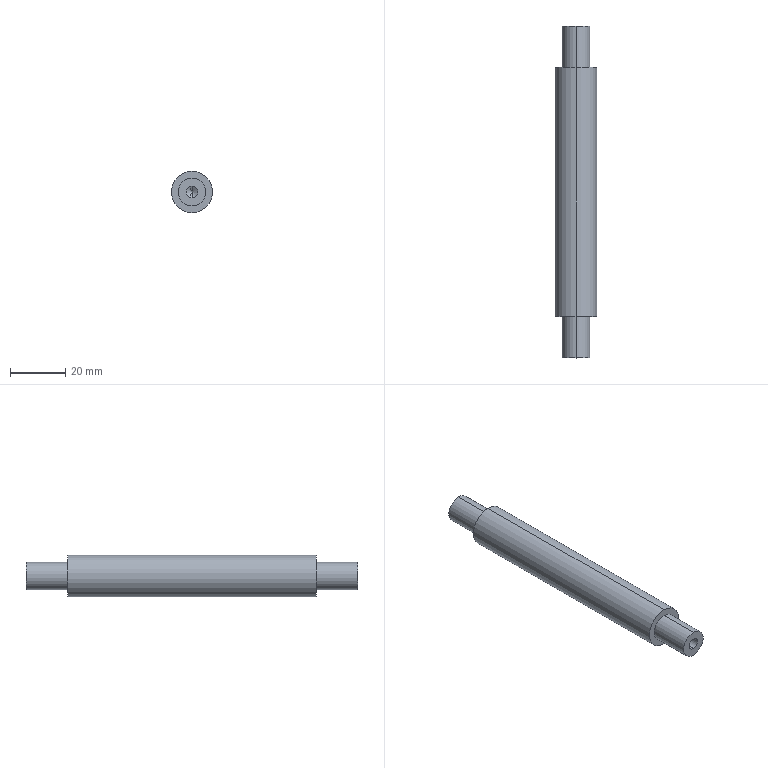Part | STEP file | PN_0006 | 1 solid | 18 faces | box 15 x 120 x 15 mm | volume 17905 mm3 | cylinder 10 | cone 4 | plane 4 | commonest cylinder face diameters 4.2 x4 10 x4 15 x2
STEP:
#1=CARTESIAN_POINT('',(0.,0.,0.));
#2=DIRECTION('',(0.,0.,1.));
#3=DIRECTION('',(1.,0.,0.));
#4=AXIS2_PLACEMENT_3D('',#1,#2,#3);
#5=CARTESIAN_POINT('',(0.,107.6,2.1));
#6=VERTEX_POINT('',#5);
#7=CARTESIAN_POINT('',(0.,120.,2.1));
#8=VERTEX_POINT('',#7);
#9=CARTESIAN_POINT('',(0.,120.,2.1));
#10=DIRECTION('',(0.,1.,0.));
#11=VECTOR('',#10,1.);
#12=LINE('',#9,#11);
#13=CARTESIAN_POINT('',(0.,120.,0.));
#14=DIRECTION('',(0.,1.,0.));
#15=DIRECTION('',(0.,0.,1.));
#16=AXIS2_PLACEMENT_3D('',#13,#14,#15);
#17=CYLINDRICAL_SURFACE('',#16,2.1);
#18=CARTESIAN_POINT('',(6.283,0.));
#19=DIRECTION('',(0.,1.));
#20=VECTOR('',#19,1.);
#21=LINE('',#18,#20);
#22=(GEOMETRIC_REPRESENTATION_CONTEXT(2)PARAMETRIC_REPRESENTATION_CONTEXT()REPRESENTATION_CONTEXT('',''));
#23=DEFINITIONAL_REPRESENTATION('',(#21),#22);
#24=PCURVE('',#17,#23);
#25=CARTESIAN_POINT('',(0.,120.,0.));
#26=DIRECTION('',(0.,1.,0.));
#27=DIRECTION('',(0.,0.,1.));
#28=AXIS2_PLACEMENT_3D('',#25,#26,#27);
#29=CYLINDRICAL_SURFACE('',#28,2.1);
#30=CARTESIAN_POINT('',(0.,0.));
#31=DIRECTION('',(0.,1.));
#32=VECTOR('',#31,1.);
#33=LINE('',#30,#32);
#34=(GEOMETRIC_REPRESENTATION_CONTEXT(2)PARAMETRIC_REPRESENTATION_CONTEXT()REPRESENTATION_CONTEXT('',''));
#35=DEFINITIONAL_REPRESENTATION('',(#33),#34);
#36=PCURVE('',#29,#35);
#37=SURFACE_CURVE('',#12,(#24,#36),.PCURVE_S1.);
#38=EDGE_CURVE('',#6,#8,#37,.T.);
#39=ORIENTED_EDGE('',*,*,#38,.T.);
#40=CARTESIAN_POINT('',(0.,120.,-2.1));
#41=VERTEX_POINT('',#40);
#42=CARTESIAN_POINT('',(0.,120.,0.));
#43=DIRECTION('',(0.,1.,0.));
#44=DIRECTION('',(0.,0.,1.));
#45=AXIS2_PLACEMENT_3D('',#42,#43,#44);
#46=CIRCLE('',#45,2.1);
#47=CARTESIAN_POINT('',(0.,0.));
#48=DIRECTION('',(1.,0.));
#49=VECTOR('',#48,1.);
#50=LINE('',#47,#49);
#51=(GEOMETRIC_REPRESENTATION_CONTEXT(2)PARAMETRIC_REPRESENTATION_CONTEXT()REPRESENTATION_CONTEXT('',''));
#52=DEFINITIONAL_REPRESENTATION('',(#50),#51);
#53=PCURVE('',#17,#52);
#54=CARTESIAN_POINT('',(0.,120.,0.));
#55=DIRECTION('',(0.,1.,0.));
#56=DIRECTION('',(0.,0.,1.));
#57=AXIS2_PLACEMENT_3D('',#54,#55,#56);
#58=PLANE('',#57);
#59=CARTESIAN_POINT('',(0.,0.));
#60=DIRECTION('',(1.,0.));
#61=AXIS2_PLACEMENT_2D('',#59,#60);
#62=CIRCLE('',#61,2.1);
#63=(GEOMETRIC_REPRESENTATION_CONTEXT(2)PARAMETRIC_REPRESENTATION_CONTEXT()REPRESENTATION_CONTEXT('',''));
#64=DEFINITIONAL_REPRESENTATION('',(#62),#63);
#65=PCURVE('',#58,#64);
#66=SURFACE_CURVE('',#46,(#53,#65),.PCURVE_S1.);
#67=EDGE_CURVE('',#41,#8,#66,.T.);
#68=ORIENTED_EDGE('',*,*,#67,.F.);
#69=CARTESIAN_POINT('',(0.,107.6,-2.1));
#70=VERTEX_POINT('',#69);
#71=CARTESIAN_POINT('',(0.,120.,-2.1));
#72=DIRECTION('',(0.,1.,0.));
#73=VECTOR('',#72,1.);
#74=LINE('',#71,#73);
#75=CARTESIAN_POINT('',(3.142,0.));
#76=DIRECTION('',(0.,1.));
#77=VECTOR('',#76,1.);
#78=LINE('',#75,#77);
#79=(GEOMETRIC_REPRESENTATION_CONTEXT(2)PARAMETRIC_REPRESENTATION_CONTEXT()REPRESENTATION_CONTEXT('',''));
#80=DEFINITIONAL_REPRESENTATION('',(#78),#79);
#81=PCURVE('',#17,#80);
#82=CARTESIAN_POINT('',(3.142,0.));
#83=DIRECTION('',(0.,1.));
#84=VECTOR('',#83,1.);
#85=LINE('',#82,#84);
#86=(GEOMETRIC_REPRESENTATION_CONTEXT(2)PARAMETRIC_REPRESENTATION_CONTEXT()REPRESENTATION_CONTEXT('',''));
#87=DEFINITIONAL_REPRESENTATION('',(#85),#86);
#88=PCURVE('',#29,#87);
#89=SURFACE_CURVE('',#74,(#81,#88),.PCURVE_S1.);
#90=EDGE_CURVE('',#70,#41,#89,.T.);
#91=ORIENTED_EDGE('',*,*,#90,.F.);
#92=CARTESIAN_POINT('',(0.,107.6,0.));
#93=DIRECTION('',(0.,1.,0.));
#94=DIRECTION('',(0.,0.,1.));
#95=AXIS2_PLACEMENT_3D('',#92,#93,#94);
#96=CIRCLE('',#95,2.1);
#97=CARTESIAN_POINT('',(0.,-12.4));
#98=DIRECTION('',(1.,0.));
#99=VECTOR('',#98,1.);
#100=LINE('',#97,#99);
#101=(GEOMETRIC_REPRESENTATION_CONTEXT(2)PARAMETRIC_REPRESENTATION_CONTEXT()REPRESENTATION_CONTEXT('',''));
#102=DEFINITIONAL_REPRESENTATION('',(#100),#101);
#103=PCURVE('',#17,#102);
#104=CARTESIAN_POINT('',(0.,107.6,0.));
#105=DIRECTION('',(0.,1.,0.));
#106=DIRECTION('',(0.,0.,1.));
#107=AXIS2_PLACEMENT_3D('',#104,#105,#106);
#108=CONICAL_SURFACE('',#107,2.1,1.03);
#109=CARTESIAN_POINT('',(0.,0.));
#110=DIRECTION('',(1.,0.));
#111=VECTOR('',#110,1.);
#112=LINE('',#109,#111);
#113=(GEOMETRIC_REPRESENTATION_CONTEXT(2)PARAMETRIC_REPRESENTATION_CONTEXT()REPRESENTATION_CONTEXT('',''));
#114=DEFINITIONAL_REPRESENTATION('',(#112),#113);
#115=PCURVE('',#108,#114);
#116=SURFACE_CURVE('',#96,(#103,#115),.PCURVE_S1.);
#117=EDGE_CURVE('',#70,#6,#116,.T.);
#118=ORIENTED_EDGE('',*,*,#117,.T.);
#119=EDGE_LOOP('',(#39,#68,#91,#118));
#120=FACE_BOUND('',#119,.F.);
#121=ADVANCED_FACE('',(#120),#17,.F.);
#122=ORIENTED_EDGE('',*,*,#117,.F.);
#123=CARTESIAN_POINT('',(0.,106.338,0.));
#124=VERTEX_POINT('',#123);
#125=CARTESIAN_POINT('',(0.,107.6,-2.1));
#126=DIRECTION('',(0.,0.515,-0.8572));
#127=VECTOR('',#126,1.);
#128=LINE('',#125,#127);
#129=CARTESIAN_POINT('',(3.142,0.));
#130=DIRECTION('',(0.,1.));
#131=VECTOR('',#130,1.);
#132=LINE('',#129,#131);
#133=(GEOMETRIC_REPRESENTATION_CONTEXT(2)PARAMETRIC_REPRESENTATION_CONTEXT()REPRESENTATION_CONTEXT('',''));
#134=DEFINITIONAL_REPRESENTATION('',(#132),#133);
#135=PCURVE('',#108,#134);
#136=CARTESIAN_POINT('',(0.,107.6,0.));
#137=DIRECTION('',(0.,1.,0.));
#138=DIRECTION('',(0.,0.,1.));
#139=AXIS2_PLACEMENT_3D('',#136,#137,#138);
#140=CONICAL_SURFACE('',#139,2.1,1.03);
#141=CARTESIAN_POINT('',(3.142,0.));
#142=DIRECTION('',(0.,1.));
#143=VECTOR('',#142,1.);
#144=LINE('',#141,#143);
#145=(GEOMETRIC_REPRESENTATION_CONTEXT(2)PARAMETRIC_REPRESENTATION_CONTEXT()REPRESENTATION_CONTEXT('',''));
#146=DEFINITIONAL_REPRESENTATION('',(#144),#145);
#147=PCURVE('',#140,#146);
#148=SURFACE_CURVE('',#128,(#135,#147),.PCURVE_S1.);
#149=EDGE_CURVE('',#124,#70,#148,.T.);
#150=ORIENTED_EDGE('',*,*,#149,.F.);
#151=CARTESIAN_POINT('',(0.,107.6,2.1));
#152=DIRECTION('',(0.,0.515,0.8572));
#153=VECTOR('',#152,1.);
#154=LINE('',#151,#153);
#155=CARTESIAN_POINT('',(6.283,0.));
#156=DIRECTION('',(0.,1.));
#157=VECTOR('',#156,1.);
#158=LINE('',#155,#157);
#159=(GEOMETRIC_REPRESENTATION_CONTEXT(2)PARAMETRIC_REPRESENTATION_CONTEXT()REPRESENTATION_CONTEXT('',''));
#160=DEFINITIONAL_REPRESENTATION('',(#158),#159);
#161=PCURVE('',#108,#160);
#162=CARTESIAN_POINT('',(0.,0.));
#163=DIRECTION('',(0.,1.));
#164=VECTOR('',#163,1.);
#165=LINE('',#162,#164);
#166=(GEOMETRIC_REPRESENTATION_CONTEXT(2)PARAMETRIC_REPRESENTATION_CONTEXT()REPRESENTATION_CONTEXT('',''));
#167=DEFINITIONAL_REPRESENTATION('',(#165),#166);
#168=PCURVE('',#140,#167);
#169=SURFACE_CURVE('',#154,(#161,#168),.PCURVE_S1.);
#170=EDGE_CURVE('',#124,#6,#169,.T.);
#171=ORIENTED_EDGE('',*,*,#170,.T.);
#172=EDGE_LOOP('',(#122,#150,#171));
#173=FACE_BOUND('',#172,.F.);
#174=ADVANCED_FACE('',(#173),#108,.F.);
#175=CARTESIAN_POINT('',(0.,12.4,-2.1));
#176=VERTEX_POINT('',#175);
#177=CARTESIAN_POINT('',(0.,0.,-2.1));
#178=VERTEX_POINT('',#177);
#179=CARTESIAN_POINT('',(0.,0.,-2.1));
#180=DIRECTION('',(0.,-1.,0.));
#181=VECTOR('',#180,1.);
#182=LINE('',#179,#181);
#183=CARTESIAN_POINT('',(0.,0.,0.));
#184=DIRECTION('',(0.,-1.,0.));
#185=DIRECTION('',(0.,0.,-1.));
#186=AXIS2_PLACEMENT_3D('',#183,#184,#185);
#187=CYLINDRICAL_SURFACE('',#186,2.1);
#188=CARTESIAN_POINT('',(6.283,0.));
#189=DIRECTION('',(0.,1.));
#190=VECTOR('',#189,1.);
#191=LINE('',#188,#190);
#192=(GEOMETRIC_REPRESENTATION_CONTEXT(2)PARAMETRIC_REPRESENTATION_CONTEXT()REPRESENTATION_CONTEXT('',''));
#193=DEFINITIONAL_REPRESENTATION('',(#191),#192);
#194=PCURVE('',#187,#193);
#195=CARTESIAN_POINT('',(0.,0.,0.));
#196=DIRECTION('',(0.,-1.,0.));
#197=DIRECTION('',(0.,0.,-1.));
#198=AXIS2_PLACEMENT_3D('',#195,#196,#197);
#199=CYLINDRICAL_SURFACE('',#198,2.1);
#200=CARTESIAN_POINT('',(0.,0.));
#201=DIRECTION('',(0.,1.));
#202=VECTOR('',#201,1.);
#203=LINE('',#200,#202);
#204=(GEOMETRIC_REPRESENTATION_CONTEXT(2)PARAMETRIC_REPRESENTATION_CONTEXT()REPRESENTATION_CONTEXT('',''));
#205=DEFINITIONAL_REPRESENTATION('',(#203),#204);
#206=PCURVE('',#199,#205);
#207=SURFACE_CURVE('',#182,(#194,#206),.PCURVE_S1.);
#208=EDGE_CURVE('',#176,#178,#207,.T.);
#209=ORIENTED_EDGE('',*,*,#208,.T.);
#210=CARTESIAN_POINT('',(0.,0.,2.1));
#211=VERTEX_POINT('',#210);
#212=CARTESIAN_POINT('',(0.,0.,0.));
#213=DIRECTION('',(0.,-1.,0.));
#214=DIRECTION('',(0.,0.,-1.));
#215=AXIS2_PLACEMENT_3D('',#212,#213,#214);
#216=CIRCLE('',#215,2.1);
#217=CARTESIAN_POINT('',(0.,0.));
#218=DIRECTION('',(1.,0.));
#219=VECTOR('',#218,1.);
#220=LINE('',#217,#219);
#221=(GEOMETRIC_REPRESENTATION_CONTEXT(2)PARAMETRIC_REPRESENTATION_CONTEXT()REPRESENTATION_CONTEXT('',''));
#222=DEFINITIONAL_REPRESENTATION('',(#220),#221);
#223=PCURVE('',#187,#222);
#224=CARTESIAN_POINT('',(0.,0.,0.));
#225=DIRECTION('',(0.,-1.,0.));
#226=DIRECTION('',(0.,0.,-1.));
#227=AXIS2_PLACEMENT_3D('',#224,#225,#226);
#228=PLANE('',#227);
#229=CARTESIAN_POINT('',(0.,0.));
#230=DIRECTION('',(1.,0.));
#231=AXIS2_PLACEMENT_2D('',#229,#230);
#232=CIRCLE('',#231,2.1);
#233=(GEOMETRIC_REPRESENTATION_CONTEXT(2)PARAMETRIC_REPRESENTATION_CONTEXT()REPRESENTATION_CONTEXT('',''));
#234=DEFINITIONAL_REPRESENTATION('',(#232),#233);
#235=PCURVE('',#228,#234);
#236=SURFACE_CURVE('',#216,(#223,#235),.PCURVE_S1.);
#237=EDGE_CURVE('',#211,#178,#236,.T.);
#238=ORIENTED_EDGE('',*,*,#237,.F.);
#239=CARTESIAN_POINT('',(0.,12.4,2.1));
#240=VERTEX_POINT('',#239);
#241=CARTESIAN_POINT('',(0.,0.,2.1));
#242=DIRECTION('',(0.,-1.,0.));
#243=VECTOR('',#242,1.);
#244=LINE('',#241,#243);
#245=CARTESIAN_POINT('',(3.142,0.));
#246=DIRECTION('',(0.,1.));
#247=VECTOR('',#246,1.);
#248=LINE('',#245,#247);
#249=(GEOMETRIC_REPRESENTATION_CONTEXT(2)PARAMETRIC_REPRESENTATION_CONTEXT()REPRESENTATION_CONTEXT('',''));
#250=DEFINITIONAL_REPRESENTATION('',(#248),#249);
#251=PCURVE('',#187,#250);
#252=CARTESIAN_POINT('',(3.142,0.));
#253=DIRECTION('',(0.,1.));
#254=VECTOR('',#253,1.);
#255=LINE('',#252,#254);
#256=(GEOMETRIC_REPRESENTATION_CONTEXT(2)PARAMETRIC_REPRESENTATION_CONTEXT()REPRESENTATION_CONTEXT('',''));
#257=DEFINITIONAL_REPRESENTATION('',(#255),#256);
#258=PCURVE('',#199,#257);
#259=SURFACE_CURVE('',#244,(#251,#258),.PCURVE_S1.);
#260=EDGE_CURVE('',#240,#211,#259,.T.);
#261=ORIENTED_EDGE('',*,*,#260,.F.);
#262=CARTESIAN_POINT('',(0.,12.4,0.));
#263=DIRECTION('',(0.,-1.,0.));
#264=DIRECTION('',(0.,0.,-1.));
#265=AXIS2_PLACEMENT_3D('',#262,#263,#264);
#266=CIRCLE('',#265,2.1);
#267=CARTESIAN_POINT('',(0.,-12.4));
#268=DIRECTION('',(1.,0.));
#269=VECTOR('',#268,1.);
#270=LINE('',#267,#269);
#271=(GEOMETRIC_REPRESENTATION_CONTEXT(2)PARAMETRIC_REPRESENTATION_CONTEXT()REPRESENTATION_CONTEXT('',''));
#272=DEFINITIONAL_REPRESENTATION('',(#270),#271);
#273=PCURVE('',#187,#272);
#274=CARTESIAN_POINT('',(0.,12.4,0.));
#275=DIRECTION('',(0.,-1.,0.));
#276=DIRECTION('',(0.,0.,-1.));
#277=AXIS2_PLACEMENT_3D('',#274,#275,#276);
#278=CONICAL_SURFACE('',#277,2.1,1.03);
#279=CARTESIAN_POINT('',(0.,0.));
#280=DIRECTION('',(1.,0.));
#281=VECTOR('',#280,1.);
#282=LINE('',#279,#281);
#283=(GEOMETRIC_REPRESENTATION_CONTEXT(2)PARAMETRIC_REPRESENTATION_CONTEXT()REPRESENTATION_CONTEXT('',''));
#284=DEFINITIONAL_REPRESENTATION('',(#282),#283);
#285=PCURVE('',#278,#284);
#286=SURFACE_CURVE('',#266,(#273,#285),.PCURVE_S1.);
#287=EDGE_CURVE('',#240,#176,#286,.T.);
#288=ORIENTED_EDGE('',*,*,#287,.T.);
#289=EDGE_LOOP('',(#209,#238,#261,#288));
#290=FACE_BOUND('',#289,.F.);
#291=ADVANCED_FACE('',(#290),#187,.F.);
#292=ORIENTED_EDGE('',*,*,#287,.F.);
#293=CARTESIAN_POINT('',(0.,13.662,0.));
#294=VERTEX_POINT('',#293);
#295=CARTESIAN_POINT('',(0.,12.4,2.1));
#296=DIRECTION('',(0.,-0.515,0.8572));
#297=VECTOR('',#296,1.);
#298=LINE('',#295,#297);
#299=CARTESIAN_POINT('',(3.142,0.));
#300=DIRECTION('',(0.,1.));
#301=VECTOR('',#300,1.);
#302=LINE('',#299,#301);
#303=(GEOMETRIC_REPRESENTATION_CONTEXT(2)PARAMETRIC_REPRESENTATION_CONTEXT()REPRESENTATION_CONTEXT('',''));
#304=DEFINITIONAL_REPRESENTATION('',(#302),#303);
#305=PCURVE('',#278,#304);
#306=CARTESIAN_POINT('',(0.,12.4,0.));
#307=DIRECTION('',(0.,-1.,0.));
#308=DIRECTION('',(0.,0.,-1.));
#309=AXIS2_PLACEMENT_3D('',#306,#307,#308);
#310=CONICAL_SURFACE('',#309,2.1,1.03);
#311=CARTESIAN_POINT('',(3.142,0.));
#312=DIRECTION('',(0.,1.));
#313=VECTOR('',#312,1.);
#314=LINE('',#311,#313);
#315=(GEOMETRIC_REPRESENTATION_CONTEXT(2)PARAMETRIC_REPRESENTATION_CONTEXT()REPRESENTATION_CONTEXT('',''));
#316=DEFINITIONAL_REPRESENTATION('',(#314),#315);
#317=PCURVE('',#310,#316);
#318=SURFACE_CURVE('',#298,(#305,#317),.PCURVE_S1.);
#319=EDGE_CURVE('',#294,#240,#318,.T.);
#320=ORIENTED_EDGE('',*,*,#319,.F.);
#321=CARTESIAN_POINT('',(0.,12.4,-2.1));
#322=DIRECTION('',(0.,-0.515,-0.8572));
#323=VECTOR('',#322,1.);
#324=LINE('',#321,#323);
#325=CARTESIAN_POINT('',(6.283,0.));
#326=DIRECTION('',(0.,1.));
#327=VECTOR('',#326,1.);
#328=LINE('',#325,#327);
#329=(GEOMETRIC_REPRESENTATION_CONTEXT(2)PARAMETRIC_REPRESENTATION_CONTEXT()REPRESENTATION_CONTEXT('',''));
#330=DEFINITIONAL_REPRESENTATION('',(#328),#329);
#331=PCURVE('',#278,#330);
#332=CARTESIAN_POINT('',(0.,0.));
#333=DIRECTION('',(0.,1.));
#334=VECTOR('',#333,1.);
#335=LINE('',#332,#334);
#336=(GEOMETRIC_REPRESENTATION_CONTEXT(2)PARAMETRIC_REPRESENTATION_CONTEXT()REPRESENTATION_CONTEXT('',''));
#337=DEFINITIONAL_REPRESENTATION('',(#335),#336);
#338=PCURVE('',#310,#337);
#339=SURFACE_CURVE('',#324,(#331,#338),.PCURVE_S1.);
#340=EDGE_CURVE('',#294,#176,#339,.T.);
#341=ORIENTED_EDGE('',*,*,#340,.T.);
#342=EDGE_LOOP('',(#292,#320,#341));
#343=FACE_BOUND('',#342,.F.);
#344=ADVANCED_FACE('',(#343),#278,.F.);
#345=CARTESIAN_POINT('',(0.,15.,-5.));
#346=VERTEX_POINT('',#345);
#347=CARTESIAN_POINT('',(0.,15.,5.));
#348=VERTEX_POINT('',#347);
#349=CARTESIAN_POINT('',(0.,15.,0.));
#350=DIRECTION('',(0.,-1.,0.));
#351=DIRECTION('',(0.,0.,-1.));
#352=AXIS2_PLACEMENT_3D('',#349,#350,#351);
#353=CIRCLE('',#352,5.);
#354=CARTESIAN_POINT('',(0.,0.,0.));
#355=DIRECTION('',(0.,-1.,0.));
#356=DIRECTION('',(0.,0.,-1.));
#357=AXIS2_PLACEMENT_3D('',#354,#355,#356);
#358=CYLINDRICAL_SURFACE('',#357,5.);
#359=CARTESIAN_POINT('',(0.,-15.));
#360=DIRECTION('',(1.,0.));
#361=VECTOR('',#360,1.);
#362=LINE('',#359,#361);
#363=(GEOMETRIC_REPRESENTATION_CONTEXT(2)PARAMETRIC_REPRESENTATION_CONTEXT()REPRESENTATION_CONTEXT('',''));
#364=DEFINITIONAL_REPRESENTATION('',(#362),#363);
#365=PCURVE('',#358,#364);
#366=CARTESIAN_POINT('',(5.,15.,0.));
#367=DIRECTION('',(0.,-1.,0.));
#368=DIRECTION('',(0.,0.,-1.));
#369=AXIS2_PLACEMENT_3D('',#366,#367,#368);
#370=PLANE('',#369);
#371=CARTESIAN_POINT('',(0.,-5.));
#372=DIRECTION('',(1.,0.));
#373=AXIS2_PLACEMENT_2D('',#371,#372);
#374=CIRCLE('',#373,5.);
#375=(GEOMETRIC_REPRESENTATION_CONTEXT(2)PARAMETRIC_REPRESENTATION_CONTEXT()REPRESENTATION_CONTEXT('',''));
#376=DEFINITIONAL_REPRESENTATION('',(#374),#375);
#377=PCURVE('',#370,#376);
#378=SURFACE_CURVE('',#353,(#365,#377),.PCURVE_S1.);
#379=EDGE_CURVE('',#346,#348,#378,.T.);
#380=ORIENTED_EDGE('',*,*,#379,.T.);
#381=CARTESIAN_POINT('',(0.,0.,5.));
#382=VERTEX_POINT('',#381);
#383=CARTESIAN_POINT('',(0.,0.,5.));
#384=DIRECTION('',(0.,-1.,0.));
#385=VECTOR('',#384,1.);
#386=LINE('',#383,#385);
#387=CARTESIAN_POINT('',(3.142,0.));
#388=DIRECTION('',(0.,1.));
#389=VECTOR('',#388,1.);
#390=LINE('',#387,#389);
#391=(GEOMETRIC_REPRESENTATION_CONTEXT(2)PARAMETRIC_REPRESENTATION_CONTEXT()REPRESENTATION_CONTEXT('',''));
#392=DEFINITIONAL_REPRESENTATION('',(#390),#391);
#393=PCURVE('',#358,#392);
#394=CARTESIAN_POINT('',(0.,0.,0.));
#395=DIRECTION('',(0.,-1.,0.));
#396=DIRECTION('',(0.,0.,-1.));
#397=AXIS2_PLACEMENT_3D('',#394,#395,#396);
#398=CYLINDRICAL_SURFACE('',#397,5.);
#399=CARTESIAN_POINT('',(3.142,0.));
#400=DIRECTION('',(0.,1.));
#401=VECTOR('',#400,1.);
#402=LINE('',#399,#401);
#403=(GEOMETRIC_REPRESENTATION_CONTEXT(2)PARAMETRIC_REPRESENTATION_CONTEXT()REPRESENTATION_CONTEXT('',''));
#404=DEFINITIONAL_REPRESENTATION('',(#402),#403);
#405=PCURVE('',#398,#404);
#406=SURFACE_CURVE('',#386,(#393,#405),.PCURVE_S1.);
#407=EDGE_CURVE('',#348,#382,#406,.T.);
#408=ORIENTED_EDGE('',*,*,#407,.T.);
#409=CARTESIAN_POINT('',(0.,0.,-5.));
#410=VERTEX_POINT('',#409);
#411=CARTESIAN_POINT('',(0.,0.,0.));
#412=DIRECTION('',(0.,-1.,0.));
#413=DIRECTION('',(0.,0.,-1.));
#414=AXIS2_PLACEMENT_3D('',#411,#412,#413);
#415=CIRCLE('',#414,5.);
#416=CARTESIAN_POINT('',(0.,0.));
#417=DIRECTION('',(1.,0.));
#418=VECTOR('',#417,1.);
#419=LINE('',#416,#418);
#420=(GEOMETRIC_REPRESENTATION_CONTEXT(2)PARAMETRIC_REPRESENTATION_CONTEXT()REPRESENTATION_CONTEXT('',''));
#421=DEFINITIONAL_REPRESENTATION('',(#419),#420);
#422=PCURVE('',#358,#421);
#423=CARTESIAN_POINT('',(0.,0.));
#424=DIRECTION('',(1.,0.));
#425=AXIS2_PLACEMENT_2D('',#423,#424);
#426=CIRCLE('',#425,5.);
#427=(GEOMETRIC_REPRESENTATION_CONTEXT(2)PARAMETRIC_REPRESENTATION_CONTEXT()REPRESENTATION_CONTEXT('',''));
#428=DEFINITIONAL_REPRESENTATION('',(#426),#427);
#429=PCURVE('',#228,#428);
#430=SURFACE_CURVE('',#415,(#422,#429),.PCURVE_S1.);
#431=EDGE_CURVE('',#410,#382,#430,.T.);
#432=ORIENTED_EDGE('',*,*,#431,.F.);
#433=CARTESIAN_POINT('',(0.,0.,-5.));
#434=DIRECTION('',(0.,-1.,0.));
#435=VECTOR('',#434,1.);
#436=LINE('',#433,#435);
#437=CARTESIAN_POINT('',(0.,0.));
#438=DIRECTION('',(0.,1.));
#439=VECTOR('',#438,1.);
#440=LINE('',#437,#439);
#441=(GEOMETRIC_REPRESENTATION_CONTEXT(2)PARAMETRIC_REPRESENTATION_CONTEXT()REPRESENTATION_CONTEXT('',''));
#442=DEFINITIONAL_REPRESENTATION('',(#440),#441);
#443=PCURVE('',#358,#442);
#444=CARTESIAN_POINT('',(6.283,0.));
#445=DIRECTION('',(0.,1.));
#446=VECTOR('',#445,1.);
#447=LINE('',#444,#446);
#448=(GEOMETRIC_REPRESENTATION_CONTEXT(2)PARAMETRIC_REPRESENTATION_CONTEXT()REPRESENTATION_CONTEXT('',''));
#449=DEFINITIONAL_REPRESENTATION('',(#447),#448);
#450=PCURVE('',#398,#449);
#451=SURFACE_CURVE('',#436,(#443,#450),.PCURVE_S1.);
#452=EDGE_CURVE('',#346,#410,#451,.T.);
#453=ORIENTED_EDGE('',*,*,#452,.F.);
#454=EDGE_LOOP('',(#380,#408,#432,#453));
#455=FACE_BOUND('',#454,.T.);
#456=ADVANCED_FACE('',(#455),#358,.T.);
#457=CARTESIAN_POINT('',(0.,105.,-7.5));
#458=VERTEX_POINT('',#457);
#459=CARTESIAN_POINT('',(0.,105.,7.5));
#460=VERTEX_POINT('',#459);
#461=CARTESIAN_POINT('',(0.,105.,0.));
#462=DIRECTION('',(0.,-1.,0.));
#463=DIRECTION('',(0.,0.,-1.));
#464=AXIS2_PLACEMENT_3D('',#461,#462,#463);
#465=CIRCLE('',#464,7.5);
#466=CARTESIAN_POINT('',(0.,0.,0.));
#467=DIRECTION('',(0.,-1.,0.));
#468=DIRECTION('',(0.,0.,-1.));
#469=AXIS2_PLACEMENT_3D('',#466,#467,#468);
#470=CYLINDRICAL_SURFACE('',#469,7.5);
#471=CARTESIAN_POINT('',(0.,-105.));
#472=DIRECTION('',(1.,0.));
#473=VECTOR('',#472,1.);
#474=LINE('',#471,#473);
#475=(GEOMETRIC_REPRESENTATION_CONTEXT(2)PARAMETRIC_REPRESENTATION_CONTEXT()REPRESENTATION_CONTEXT('',''));
#476=DEFINITIONAL_REPRESENTATION('',(#474),#475);
#477=PCURVE('',#470,#476);
#478=CARTESIAN_POINT('',(5.,105.,0.));
#479=DIRECTION('',(0.,1.,0.));
#480=DIRECTION('',(0.,0.,1.));
#481=AXIS2_PLACEMENT_3D('',#478,#479,#480);
#482=PLANE('',#481);
#483=CARTESIAN_POINT('',(-7.5,-5.));
#484=CARTESIAN_POINT('',(-7.5,7.99));
#485=CARTESIAN_POINT('',(3.75,1.495));
#486=CARTESIAN_POINT('',(15.,-5.));
#487=CARTESIAN_POINT('',(3.75,-11.495));
#488=CARTESIAN_POINT('',(-7.5,-17.99));
#489=CARTESIAN_POINT('',(-7.5,-5.));
#490=(BOUNDED_CURVE()B_SPLINE_CURVE(2,(#483,#484,#485,#486,#487,#488,#489),.UNSPECIFIED.,.T.,.F.)B_SPLINE_CURVE_WITH_KNOTS((1,2,2,2,2,1),(-2.094,0.,2.094,4.189,6.283,8.378),.UNSPECIFIED.)CURVE()GEOMETRIC_REPRESENTATION_ITEM()RATIONAL_B_SPLINE_CURVE((1.,0.5,1.,0.5,1.,0.5,1.))REPRESENTATION_ITEM(''));
#491=(GEOMETRIC_REPRESENTATION_CONTEXT(2)PARAMETRIC_REPRESENTATION_CONTEXT()REPRESENTATION_CONTEXT('',''));
#492=DEFINITIONAL_REPRESENTATION('',(#490),#491);
#493=PCURVE('',#482,#492);
#494=SURFACE_CURVE('',#465,(#477,#493),.PCURVE_S1.);
#495=EDGE_CURVE('',#458,#460,#494,.T.);
#496=ORIENTED_EDGE('',*,*,#495,.T.);
#497=CARTESIAN_POINT('',(0.,15.,7.5));
#498=VERTEX_POINT('',#497);
#499=CARTESIAN_POINT('',(0.,0.,7.5));
#500=DIRECTION('',(0.,-1.,0.));
#501=VECTOR('',#500,1.);
#502=LINE('',#499,#501);
#503=CARTESIAN_POINT('',(3.142,0.));
#504=DIRECTION('',(0.,1.));
#505=VECTOR('',#504,1.);
#506=LINE('',#503,#505);
#507=(GEOMETRIC_REPRESENTATION_CONTEXT(2)PARAMETRIC_REPRESENTATION_CONTEXT()REPRESENTATION_CONTEXT('',''));
#508=DEFINITIONAL_REPRESENTATION('',(#506),#507);
#509=PCURVE('',#470,#508);
#510=CARTESIAN_POINT('',(0.,0.,0.));
#511=DIRECTION('',(0.,-1.,0.));
#512=DIRECTION('',(0.,0.,-1.));
#513=AXIS2_PLACEMENT_3D('',#510,#511,#512);
#514=CYLINDRICAL_SURFACE('',#513,7.5);
#515=CARTESIAN_POINT('',(3.142,0.));
#516=DIRECTION('',(0.,1.));
#517=VECTOR('',#516,1.);
#518=LINE('',#515,#517);
#519=(GEOMETRIC_REPRESENTATION_CONTEXT(2)PARAMETRIC_REPRESENTATION_CONTEXT()REPRESENTATION_CONTEXT('',''));
#520=DEFINITIONAL_REPRESENTATION('',(#518),#519);
#521=PCURVE('',#514,#520);
#522=SURFACE_CURVE('',#502,(#509,#521),.PCURVE_S1.);
#523=EDGE_CURVE('',#460,#498,#522,.T.);
#524=ORIENTED_EDGE('',*,*,#523,.T.);
#525=CARTESIAN_POINT('',(0.,15.,-7.5));
#526=VERTEX_POINT('',#525);
#527=CARTESIAN_POINT('',(0.,15.,0.));
#528=DIRECTION('',(0.,-1.,0.));
#529=DIRECTION('',(0.,0.,-1.));
#530=AXIS2_PLACEMENT_3D('',#527,#528,#529);
#531=CIRCLE('',#530,7.5);
#532=CARTESIAN_POINT('',(0.,-15.));
#533=DIRECTION('',(1.,0.));
#534=VECTOR('',#533,1.);
#535=LINE('',#532,#534);
#536=(GEOMETRIC_REPRESENTATION_CONTEXT(2)PARAMETRIC_REPRESENTATION_CONTEXT()REPRESENTATION_CONTEXT('',''));
#537=DEFINITIONAL_REPRESENTATION('',(#535),#536);
#538=PCURVE('',#470,#537);
#539=CARTESIAN_POINT('',(0.,-5.));
#540=DIRECTION('',(1.,0.));
#541=AXIS2_PLACEMENT_2D('',#539,#540);
#542=CIRCLE('',#541,7.5);
#543=(GEOMETRIC_REPRESENTATION_CONTEXT(2)PARAMETRIC_REPRESENTATION_CONTEXT()REPRESENTATION_CONTEXT('',''));
#544=DEFINITIONAL_REPRESENTATION('',(#542),#543);
#545=PCURVE('',#370,#544);
#546=SURFACE_CURVE('',#531,(#538,#545),.PCURVE_S1.);
#547=EDGE_CURVE('',#526,#498,#546,.T.);
#548=ORIENTED_EDGE('',*,*,#547,.F.);
#549=CARTESIAN_POINT('',(0.,0.,-7.5));
#550=DIRECTION('',(0.,-1.,0.));
#551=VECTOR('',#550,1.);
#552=LINE('',#549,#551);
#553=CARTESIAN_POINT('',(0.,0.));
#554=DIRECTION('',(0.,1.));
#555=VECTOR('',#554,1.);
#556=LINE('',#553,#555);
#557=(GEOMETRIC_REPRESENTATION_CONTEXT(2)PARAMETRIC_REPRESENTATION_CONTEXT()REPRESENTATION_CONTEXT('',''));
#558=DEFINITIONAL_REPRESENTATION('',(#556),#557);
#559=PCURVE('',#470,#558);
#560=CARTESIAN_POINT('',(6.283,0.));
#561=DIRECTION('',(0.,1.));
#562=VECTOR('',#561,1.);
#563=LINE('',#560,#562);
#564=(GEOMETRIC_REPRESENTATION_CONTEXT(2)PARAMETRIC_REPRESENTATION_CONTEXT()REPRESENTATION_CONTEXT('',''));
#565=DEFINITIONAL_REPRESENTATION('',(#563),#564);
#566=PCURVE('',#514,#565);
#567=SURFACE_CURVE('',#552,(#559,#566),.PCURVE_S1.);
#568=EDGE_CURVE('',#458,#526,#567,.T.);
#569=ORIENTED_EDGE('',*,*,#568,.F.);
#570=EDGE_LOOP('',(#496,#524,#548,#569));
#571=FACE_BOUND('',#570,.T.);
#572=ADVANCED_FACE('',(#571),#470,.T.);
#573=CARTESIAN_POINT('',(0.,120.,-5.));
#574=VERTEX_POINT('',#573);
#575=CARTESIAN_POINT('',(0.,120.,5.));
#576=VERTEX_POINT('',#575);
#577=CARTESIAN_POINT('',(0.,120.,0.));
#578=DIRECTION('',(0.,-1.,0.));
#579=DIRECTION('',(0.,0.,-1.));
#580=AXIS2_PLACEMENT_3D('',#577,#578,#579);
#581=CIRCLE('',#580,5.);
#582=CARTESIAN_POINT('',(0.,0.,0.));
#583=DIRECTION('',(0.,-1.,0.));
#584=DIRECTION('',(0.,0.,-1.));
#585=AXIS2_PLACEMENT_3D('',#582,#583,#584);
#586=CYLINDRICAL_SURFACE('',#585,5.);
#587=CARTESIAN_POINT('',(0.,-120.));
#588=DIRECTION('',(1.,0.));
#589=VECTOR('',#588,1.);
#590=LINE('',#587,#589);
#591=(GEOMETRIC_REPRESENTATION_CONTEXT(2)PARAMETRIC_REPRESENTATION_CONTEXT()REPRESENTATION_CONTEXT('',''));
#592=DEFINITIONAL_REPRESENTATION('',(#590),#591);
#593=PCURVE('',#586,#592);
#594=CARTESIAN_POINT('',(-5.,0.));
#595=CARTESIAN_POINT('',(-5.,8.66));
#596=CARTESIAN_POINT('',(2.5,4.33));
#597=CARTESIAN_POINT('',(10.,0.));
#598=CARTESIAN_POINT('',(2.5,-4.33));
#599=CARTESIAN_POINT('',(-5.,-8.66));
#600=CARTESIAN_POINT('',(-5.,0.));
#601=(BOUNDED_CURVE()B_SPLINE_CURVE(2,(#594,#595,#596,#597,#598,#599,#600),.UNSPECIFIED.,.T.,.F.)B_SPLINE_CURVE_WITH_KNOTS((1,2,2,2,2,1),(-2.094,0.,2.094,4.189,6.283,8.378),.UNSPECIFIED.)CURVE()GEOMETRIC_REPRESENTATION_ITEM()RATIONAL_B_SPLINE_CURVE((1.,0.5,1.,0.5,1.,0.5,1.))REPRESENTATION_ITEM(''));
#602=(GEOMETRIC_REPRESENTATION_CONTEXT(2)PARAMETRIC_REPRESENTATION_CONTEXT()REPRESENTATION_CONTEXT('',''));
#603=DEFINITIONAL_REPRESENTATION('',(#601),#602);
#604=PCURVE('',#58,#603);
#605=SURFACE_CURVE('',#581,(#593,#604),.PCURVE_S1.);
#606=EDGE_CURVE('',#574,#576,#605,.T.);
#607=ORIENTED_EDGE('',*,*,#606,.T.);
#608=CARTESIAN_POINT('',(0.,105.,5.));
#609=VERTEX_POINT('',#608);
#610=CARTESIAN_POINT('',(0.,0.,5.));
#611=DIRECTION('',(0.,-1.,0.));
#612=VECTOR('',#611,1.);
#613=LINE('',#610,#612);
#614=CARTESIAN_POINT('',(3.142,0.));
#615=DIRECTION('',(0.,1.));
#616=VECTOR('',#615,1.);
#617=LINE('',#614,#616);
#618=(GEOMETRIC_REPRESENTATION_CONTEXT(2)PARAMETRIC_REPRESENTATION_CONTEXT()REPRESENTATION_CONTEXT('',''));
#619=DEFINITIONAL_REPRESENTATION('',(#617),#618);
#620=PCURVE('',#586,#619);
#621=CARTESIAN_POINT('',(0.,0.,0.));
#622=DIRECTION('',(0.,-1.,0.));
#623=DIRECTION('',(0.,0.,-1.));
#624=AXIS2_PLACEMENT_3D('',#621,#622,#623);
#625=CYLINDRICAL_SURFACE('',#624,5.);
#626=CARTESIAN_POINT('',(3.142,0.));
#627=DIRECTION('',(0.,1.));
#628=VECTOR('',#627,1.);
#629=LINE('',#626,#628);
#630=(GEOMETRIC_REPRESENTATION_CONTEXT(2)PARAMETRIC_REPRESENTATION_CONTEXT()REPRESENTATION_CONTEXT('',''));
#631=DEFINITIONAL_REPRESENTATION('',(#629),#630);
#632=PCURVE('',#625,#631);
#633=SURFACE_CURVE('',#613,(#620,#632),.PCURVE_S1.);
#634=EDGE_CURVE('',#576,#609,#633,.T.);
#635=ORIENTED_EDGE('',*,*,#634,.T.);
#636=CARTESIAN_POINT('',(0.,105.,-5.));
#637=VERTEX_POINT('',#636);
#638=CARTESIAN_POINT('',(0.,105.,0.));
#639=DIRECTION('',(0.,-1.,0.));
#640=DIRECTION('',(0.,0.,-1.));
#641=AXIS2_PLACEMENT_3D('',#638,#639,#640);
#642=CIRCLE('',#641,5.);
#643=CARTESIAN_POINT('',(0.,-105.));
#644=DIRECTION('',(1.,0.));
#645=VECTOR('',#644,1.);
#646=LINE('',#643,#645);
#647=(GEOMETRIC_REPRESENTATION_CONTEXT(2)PARAMETRIC_REPRESENTATION_CONTEXT()REPRESENTATION_CONTEXT('',''));
#648=DEFINITIONAL_REPRESENTATION('',(#646),#647);
#649=PCURVE('',#586,#648);
#650=CARTESIAN_POINT('',(-5.,-5.));
#651=CARTESIAN_POINT('',(-5.,3.66));
#652=CARTESIAN_POINT('',(2.5,-0.6699));
#653=CARTESIAN_POINT('',(10.,-5.));
#654=CARTESIAN_POINT('',(2.5,-9.33));
#655=CARTESIAN_POINT('',(-5.,-13.66));
#656=CARTESIAN_POINT('',(-5.,-5.));
#657=(BOUNDED_CURVE()B_SPLINE_CURVE(2,(#650,#651,#652,#653,#654,#655,#656),.UNSPECIFIED.,.T.,.F.)B_SPLINE_CURVE_WITH_KNOTS((1,2,2,2,2,1),(-2.094,0.,2.094,4.189,6.283,8.378),.UNSPECIFIED.)CURVE()GEOMETRIC_REPRESENTATION_ITEM()RATIONAL_B_SPLINE_CURVE((1.,0.5,1.,0.5,1.,0.5,1.))REPRESENTATION_ITEM(''));
#658=(GEOMETRIC_REPRESENTATION_CONTEXT(2)PARAMETRIC_REPRESENTATION_CONTEXT()REPRESENTATION_CONTEXT('',''));
#659=DEFINITIONAL_REPRESENTATION('',(#657),#658);
#660=PCURVE('',#482,#659);
#661=SURFACE_CURVE('',#642,(#649,#660),.PCURVE_S1.);
#662=EDGE_CURVE('',#637,#609,#661,.T.);
#663=ORIENTED_EDGE('',*,*,#662,.F.);
#664=CARTESIAN_POINT('',(0.,0.,-5.));
#665=DIRECTION('',(0.,-1.,0.));
#666=VECTOR('',#665,1.);
#667=LINE('',#664,#666);
#668=CARTESIAN_POINT('',(0.,0.));
#669=DIRECTION('',(0.,1.));
#670=VECTOR('',#669,1.);
#671=LINE('',#668,#670);
#672=(GEOMETRIC_REPRESENTATION_CONTEXT(2)PARAMETRIC_REPRESENTATION_CONTEXT()REPRESENTATION_CONTEXT('',''));
#673=DEFINITIONAL_REPRESENTATION('',(#671),#672);
#674=PCURVE('',#586,#673);
#675=CARTESIAN_POINT('',(6.283,0.));
#676=DIRECTION('',(0.,1.));
#677=VECTOR('',#676,1.);
#678=LINE('',#675,#677);
#679=(GEOMETRIC_REPRESENTATION_CONTEXT(2)PARAMETRIC_REPRESENTATION_CONTEXT()REPRESENTATION_CONTEXT('',''));
#680=DEFINITIONAL_REPRESENTATION('',(#678),#679);
#681=PCURVE('',#625,#680);
#682=SURFACE_CURVE('',#667,(#674,#681),.PCURVE_S1.);
#683=EDGE_CURVE('',#574,#637,#682,.T.);
#684=ORIENTED_EDGE('',*,*,#683,.F.);
#685=EDGE_LOOP('',(#607,#635,#663,#684));
#686=FACE_BOUND('',#685,.T.);
#687=ADVANCED_FACE('',(#686),#586,.T.);
#688=CARTESIAN_POINT('',(0.,120.,0.));
#689=DIRECTION('',(0.,1.,0.));
#690=DIRECTION('',(0.,0.,1.));
#691=AXIS2_PLACEMENT_3D('',#688,#689,#690);
#692=CIRCLE('',#691,2.1);
#693=CARTESIAN_POINT('',(0.,0.));
#694=DIRECTION('',(1.,0.));
#695=AXIS2_PLACEMENT_2D('',#693,#694);
#696=CIRCLE('',#695,2.1);
#697=(GEOMETRIC_REPRESENTATION_CONTEXT(2)PARAMETRIC_REPRESENTATION_CONTEXT()REPRESENTATION_CONTEXT('',''));
#698=DEFINITIONAL_REPRESENTATION('',(#696),#697);
#699=PCURVE('',#58,#698);
#700=CARTESIAN_POINT('',(0.,0.));
#701=DIRECTION('',(1.,0.));
#702=VECTOR('',#701,1.);
#703=LINE('',#700,#702);
#704=(GEOMETRIC_REPRESENTATION_CONTEXT(2)PARAMETRIC_REPRESENTATION_CONTEXT()REPRESENTATION_CONTEXT('',''));
#705=DEFINITIONAL_REPRESENTATION('',(#703),#704);
#706=PCURVE('',#29,#705);
#707=SURFACE_CURVE('',#692,(#699,#706),.PCURVE_S1.);
#708=EDGE_CURVE('',#8,#41,#707,.T.);
#709=ORIENTED_EDGE('',*,*,#708,.F.);
#710=ORIENTED_EDGE('',*,*,#67,.F.);
#711=EDGE_LOOP('',(#709,#710));
#712=FACE_BOUND('',#711,.T.);
#713=ORIENTED_EDGE('',*,*,#606,.F.);
#714=CARTESIAN_POINT('',(0.,120.,0.));
#715=DIRECTION('',(0.,-1.,0.));
#716=DIRECTION('',(0.,0.,-1.));
#717=AXIS2_PLACEMENT_3D('',#714,#715,#716);
#718=CIRCLE('',#717,5.);
#719=CARTESIAN_POINT('',(-5.,0.));
#720=CARTESIAN_POINT('',(-5.,8.66));
#721=CARTESIAN_POINT('',(2.5,4.33));
#722=CARTESIAN_POINT('',(10.,0.));
#723=CARTESIAN_POINT('',(2.5,-4.33));
#724=CARTESIAN_POINT('',(-5.,-8.66));
#725=CARTESIAN_POINT('',(-5.,0.));
#726=(BOUNDED_CURVE()B_SPLINE_CURVE(2,(#719,#720,#721,#722,#723,#724,#725),.UNSPECIFIED.,.T.,.F.)B_SPLINE_CURVE_WITH_KNOTS((1,2,2,2,2,1),(-2.094,0.,2.094,4.189,6.283,8.378),.UNSPECIFIED.)CURVE()GEOMETRIC_REPRESENTATION_ITEM()RATIONAL_B_SPLINE_CURVE((1.,0.5,1.,0.5,1.,0.5,1.))REPRESENTATION_ITEM(''));
#727=(GEOMETRIC_REPRESENTATION_CONTEXT(2)PARAMETRIC_REPRESENTATION_CONTEXT()REPRESENTATION_CONTEXT('',''));
#728=DEFINITIONAL_REPRESENTATION('',(#726),#727);
#729=PCURVE('',#58,#728);
#730=CARTESIAN_POINT('',(0.,-120.));
#731=DIRECTION('',(1.,0.));
#732=VECTOR('',#731,1.);
#733=LINE('',#730,#732);
#734=(GEOMETRIC_REPRESENTATION_CONTEXT(2)PARAMETRIC_REPRESENTATION_CONTEXT()REPRESENTATION_CONTEXT('',''));
#735=DEFINITIONAL_REPRESENTATION('',(#733),#734);
#736=PCURVE('',#625,#735);
#737=SURFACE_CURVE('',#718,(#729,#736),.PCURVE_S1.);
#738=EDGE_CURVE('',#576,#574,#737,.T.);
#739=ORIENTED_EDGE('',*,*,#738,.F.);
#740=EDGE_LOOP('',(#713,#739));
#741=FACE_BOUND('',#740,.T.);
#742=ADVANCED_FACE('',(#712,#741),#58,.T.);
#743=ORIENTED_EDGE('',*,*,#634,.F.);
#744=ORIENTED_EDGE('',*,*,#738,.T.);
#745=ORIENTED_EDGE('',*,*,#683,.T.);
#746=CARTESIAN_POINT('',(0.,105.,0.));
#747=DIRECTION('',(0.,-1.,0.));
#748=DIRECTION('',(0.,0.,-1.));
#749=AXIS2_PLACEMENT_3D('',#746,#747,#748);
#750=CIRCLE('',#749,5.);
#751=CARTESIAN_POINT('',(0.,-105.));
#752=DIRECTION('',(1.,0.));
#753=VECTOR('',#752,1.);
#754=LINE('',#751,#753);
#755=(GEOMETRIC_REPRESENTATION_CONTEXT(2)PARAMETRIC_REPRESENTATION_CONTEXT()REPRESENTATION_CONTEXT('',''));
#756=DEFINITIONAL_REPRESENTATION('',(#754),#755);
#757=PCURVE('',#625,#756);
#758=CARTESIAN_POINT('',(-5.,-5.));
#759=CARTESIAN_POINT('',(-5.,3.66));
#760=CARTESIAN_POINT('',(2.5,-0.6699));
#761=CARTESIAN_POINT('',(10.,-5.));
#762=CARTESIAN_POINT('',(2.5,-9.33));
#763=CARTESIAN_POINT('',(-5.,-13.66));
#764=CARTESIAN_POINT('',(-5.,-5.));
#765=(BOUNDED_CURVE()B_SPLINE_CURVE(2,(#758,#759,#760,#761,#762,#763,#764),.UNSPECIFIED.,.T.,.F.)B_SPLINE_CURVE_WITH_KNOTS((1,2,2,2,2,1),(-2.094,0.,2.094,4.189,6.283,8.378),.UNSPECIFIED.)CURVE()GEOMETRIC_REPRESENTATION_ITEM()RATIONAL_B_SPLINE_CURVE((1.,0.5,1.,0.5,1.,0.5,1.))REPRESENTATION_ITEM(''));
#766=(GEOMETRIC_REPRESENTATION_CONTEXT(2)PARAMETRIC_REPRESENTATION_CONTEXT()REPRESENTATION_CONTEXT('',''));
#767=DEFINITIONAL_REPRESENTATION('',(#765),#766);
#768=PCURVE('',#482,#767);
#769=SURFACE_CURVE('',#750,(#757,#768),.PCURVE_S1.);
#770=EDGE_CURVE('',#609,#637,#769,.T.);
#771=ORIENTED_EDGE('',*,*,#770,.F.);
#772=EDGE_LOOP('',(#743,#744,#745,#771));
#773=FACE_BOUND('',#772,.T.);
#774=ADVANCED_FACE('',(#773),#625,.T.);
#775=ORIENTED_EDGE('',*,*,#662,.T.);
#776=ORIENTED_EDGE('',*,*,#770,.T.);
#777=EDGE_LOOP('',(#775,#776));
#778=FACE_BOUND('',#777,.T.);
#779=ORIENTED_EDGE('',*,*,#495,.F.);
#780=CARTESIAN_POINT('',(0.,105.,0.));
#781=DIRECTION('',(0.,-1.,0.));
#782=DIRECTION('',(0.,0.,-1.));
#783=AXIS2_PLACEMENT_3D('',#780,#781,#782);
#784=CIRCLE('',#783,7.5);
#785=CARTESIAN_POINT('',(-7.5,-5.));
#786=CARTESIAN_POINT('',(-7.5,7.99));
#787=CARTESIAN_POINT('',(3.75,1.495));
#788=CARTESIAN_POINT('',(15.,-5.));
#789=CARTESIAN_POINT('',(3.75,-11.495));
#790=CARTESIAN_POINT('',(-7.5,-17.99));
#791=CARTESIAN_POINT('',(-7.5,-5.));
#792=(BOUNDED_CURVE()B_SPLINE_CURVE(2,(#785,#786,#787,#788,#789,#790,#791),.UNSPECIFIED.,.T.,.F.)B_SPLINE_CURVE_WITH_KNOTS((1,2,2,2,2,1),(-2.094,0.,2.094,4.189,6.283,8.378),.UNSPECIFIED.)CURVE()GEOMETRIC_REPRESENTATION_ITEM()RATIONAL_B_SPLINE_CURVE((1.,0.5,1.,0.5,1.,0.5,1.))REPRESENTATION_ITEM(''));
#793=(GEOMETRIC_REPRESENTATION_CONTEXT(2)PARAMETRIC_REPRESENTATION_CONTEXT()REPRESENTATION_CONTEXT('',''));
#794=DEFINITIONAL_REPRESENTATION('',(#792),#793);
#795=PCURVE('',#482,#794);
#796=CARTESIAN_POINT('',(0.,-105.));
#797=DIRECTION('',(1.,0.));
#798=VECTOR('',#797,1.);
#799=LINE('',#796,#798);
#800=(GEOMETRIC_REPRESENTATION_CONTEXT(2)PARAMETRIC_REPRESENTATION_CONTEXT()REPRESENTATION_CONTEXT('',''));
#801=DEFINITIONAL_REPRESENTATION('',(#799),#800);
#802=PCURVE('',#514,#801);
#803=SURFACE_CURVE('',#784,(#795,#802),.PCURVE_S1.);
#804=EDGE_CURVE('',#460,#458,#803,.T.);
#805=ORIENTED_EDGE('',*,*,#804,.F.);
#806=EDGE_LOOP('',(#779,#805));
#807=FACE_BOUND('',#806,.T.);
#808=ADVANCED_FACE('',(#778,#807),#482,.T.);
#809=ORIENTED_EDGE('',*,*,#523,.F.);
#810=ORIENTED_EDGE('',*,*,#804,.T.);
#811=ORIENTED_EDGE('',*,*,#568,.T.);
#812=CARTESIAN_POINT('',(0.,15.,0.));
#813=DIRECTION('',(0.,-1.,0.));
#814=DIRECTION('',(0.,0.,-1.));
#815=AXIS2_PLACEMENT_3D('',#812,#813,#814);
#816=CIRCLE('',#815,7.5);
#817=CARTESIAN_POINT('',(0.,-15.));
#818=DIRECTION('',(1.,0.));
#819=VECTOR('',#818,1.);
#820=LINE('',#817,#819);
#821=(GEOMETRIC_REPRESENTATION_CONTEXT(2)PARAMETRIC_REPRESENTATION_CONTEXT()REPRESENTATION_CONTEXT('',''));
#822=DEFINITIONAL_REPRESENTATION('',(#820),#821);
#823=PCURVE('',#514,#822);
#824=CARTESIAN_POINT('',(0.,-5.));
#825=DIRECTION('',(1.,0.));
#826=AXIS2_PLACEMENT_2D('',#824,#825);
#827=CIRCLE('',#826,7.5);
#828=(GEOMETRIC_REPRESENTATION_CONTEXT(2)PARAMETRIC_REPRESENTATION_CONTEXT()REPRESENTATION_CONTEXT('',''));
#829=DEFINITIONAL_REPRESENTATION('',(#827),#828);
#830=PCURVE('',#370,#829);
#831=SURFACE_CURVE('',#816,(#823,#830),.PCURVE_S1.);
#832=EDGE_CURVE('',#498,#526,#831,.T.);
#833=ORIENTED_EDGE('',*,*,#832,.F.);
#834=EDGE_LOOP('',(#809,#810,#811,#833));
#835=FACE_BOUND('',#834,.T.);
#836=ADVANCED_FACE('',(#835),#514,.T.);
#837=ORIENTED_EDGE('',*,*,#547,.T.);
#838=ORIENTED_EDGE('',*,*,#832,.T.);
#839=EDGE_LOOP('',(#837,#838));
#840=FACE_BOUND('',#839,.T.);
#841=ORIENTED_EDGE('',*,*,#379,.F.);
#842=CARTESIAN_POINT('',(0.,15.,0.));
#843=DIRECTION('',(0.,-1.,0.));
#844=DIRECTION('',(0.,0.,-1.));
#845=AXIS2_PLACEMENT_3D('',#842,#843,#844);
#846=CIRCLE('',#845,5.);
#847=CARTESIAN_POINT('',(0.,-5.));
#848=DIRECTION('',(1.,0.));
#849=AXIS2_PLACEMENT_2D('',#847,#848);
#850=CIRCLE('',#849,5.);
#851=(GEOMETRIC_REPRESENTATION_CONTEXT(2)PARAMETRIC_REPRESENTATION_CONTEXT()REPRESENTATION_CONTEXT('',''));
#852=DEFINITIONAL_REPRESENTATION('',(#850),#851);
#853=PCURVE('',#370,#852);
#854=CARTESIAN_POINT('',(0.,-15.));
#855=DIRECTION('',(1.,0.));
#856=VECTOR('',#855,1.);
#857=LINE('',#854,#856);
#858=(GEOMETRIC_REPRESENTATION_CONTEXT(2)PARAMETRIC_REPRESENTATION_CONTEXT()REPRESENTATION_CONTEXT('',''));
#859=DEFINITIONAL_REPRESENTATION('',(#857),#858);
#860=PCURVE('',#398,#859);
#861=SURFACE_CURVE('',#846,(#853,#860),.PCURVE_S1.);
#862=EDGE_CURVE('',#348,#346,#861,.T.);
#863=ORIENTED_EDGE('',*,*,#862,.F.);
#864=EDGE_LOOP('',(#841,#863));
#865=FACE_BOUND('',#864,.T.);
#866=ADVANCED_FACE('',(#840,#865),#370,.T.);
#867=ORIENTED_EDGE('',*,*,#407,.F.);
#868=ORIENTED_EDGE('',*,*,#862,.T.);
#869=ORIENTED_EDGE('',*,*,#452,.T.);
#870=CARTESIAN_POINT('',(0.,0.,0.));
#871=DIRECTION('',(0.,-1.,0.));
#872=DIRECTION('',(0.,0.,-1.));
#873=AXIS2_PLACEMENT_3D('',#870,#871,#872);
#874=CIRCLE('',#873,5.);
#875=CARTESIAN_POINT('',(0.,0.));
#876=DIRECTION('',(1.,0.));
#877=VECTOR('',#876,1.);
#878=LINE('',#875,#877);
#879=(GEOMETRIC_REPRESENTATION_CONTEXT(2)PARAMETRIC_REPRESENTATION_CONTEXT()REPRESENTATION_CONTEXT('',''));
#880=DEFINITIONAL_REPRESENTATION('',(#878),#879);
#881=PCURVE('',#398,#880);
#882=CARTESIAN_POINT('',(0.,0.));
#883=DIRECTION('',(1.,0.));
#884=AXIS2_PLACEMENT_2D('',#882,#883);
#885=CIRCLE('',#884,5.);
#886=(GEOMETRIC_REPRESENTATION_CONTEXT(2)PARAMETRIC_REPRESENTATION_CONTEXT()REPRESENTATION_CONTEXT('',''));
#887=DEFINITIONAL_REPRESENTATION('',(#885),#886);
#888=PCURVE('',#228,#887);
#889=SURFACE_CURVE('',#874,(#881,#888),.PCURVE_S1.);
#890=EDGE_CURVE('',#382,#410,#889,.T.);
#891=ORIENTED_EDGE('',*,*,#890,.F.);
#892=EDGE_LOOP('',(#867,#868,#869,#891));
#893=FACE_BOUND('',#892,.T.);
#894=ADVANCED_FACE('',(#893),#398,.T.);
#895=CARTESIAN_POINT('',(0.,0.,0.));
#896=DIRECTION('',(0.,-1.,0.));
#897=DIRECTION('',(0.,0.,-1.));
#898=AXIS2_PLACEMENT_3D('',#895,#896,#897);
#899=CIRCLE('',#898,2.1);
#900=CARTESIAN_POINT('',(0.,0.));
#901=DIRECTION('',(1.,0.));
#902=AXIS2_PLACEMENT_2D('',#900,#901);
#903=CIRCLE('',#902,2.1);
#904=(GEOMETRIC_REPRESENTATION_CONTEXT(2)PARAMETRIC_REPRESENTATION_CONTEXT()REPRESENTATION_CONTEXT('',''));
#905=DEFINITIONAL_REPRESENTATION('',(#903),#904);
#906=PCURVE('',#228,#905);
#907=CARTESIAN_POINT('',(0.,0.));
#908=DIRECTION('',(1.,0.));
#909=VECTOR('',#908,1.);
#910=LINE('',#907,#909);
#911=(GEOMETRIC_REPRESENTATION_CONTEXT(2)PARAMETRIC_REPRESENTATION_CONTEXT()REPRESENTATION_CONTEXT('',''));
#912=DEFINITIONAL_REPRESENTATION('',(#910),#911);
#913=PCURVE('',#199,#912);
#914=SURFACE_CURVE('',#899,(#906,#913),.PCURVE_S1.);
#915=EDGE_CURVE('',#178,#211,#914,.T.);
#916=ORIENTED_EDGE('',*,*,#915,.F.);
#917=ORIENTED_EDGE('',*,*,#237,.F.);
#918=EDGE_LOOP('',(#916,#917));
#919=FACE_BOUND('',#918,.T.);
#920=ORIENTED_EDGE('',*,*,#431,.T.);
#921=ORIENTED_EDGE('',*,*,#890,.T.);
#922=EDGE_LOOP('',(#920,#921));
#923=FACE_BOUND('',#922,.T.);
#924=ADVANCED_FACE('',(#919,#923),#228,.T.);
#925=CARTESIAN_POINT('',(0.,12.4,0.));
#926=DIRECTION('',(0.,-1.,0.));
#927=DIRECTION('',(0.,0.,-1.));
#928=AXIS2_PLACEMENT_3D('',#925,#926,#927);
#929=CIRCLE('',#928,2.1);
#930=CARTESIAN_POINT('',(0.,0.));
#931=DIRECTION('',(1.,0.));
#932=VECTOR('',#931,1.);
#933=LINE('',#930,#932);
#934=(GEOMETRIC_REPRESENTATION_CONTEXT(2)PARAMETRIC_REPRESENTATION_CONTEXT()REPRESENTATION_CONTEXT('',''));
#935=DEFINITIONAL_REPRESENTATION('',(#933),#934);
#936=PCURVE('',#310,#935);
#937=CARTESIAN_POINT('',(0.,-12.4));
#938=DIRECTION('',(1.,0.));
#939=VECTOR('',#938,1.);
#940=LINE('',#937,#939);
#941=(GEOMETRIC_REPRESENTATION_CONTEXT(2)PARAMETRIC_REPRESENTATION_CONTEXT()REPRESENTATION_CONTEXT('',''));
#942=DEFINITIONAL_REPRESENTATION('',(#940),#941);
#943=PCURVE('',#199,#942);
#944=SURFACE_CURVE('',#929,(#936,#943),.PCURVE_S1.);
#945=EDGE_CURVE('',#176,#240,#944,.T.);
#946=ORIENTED_EDGE('',*,*,#945,.F.);
#947=ORIENTED_EDGE('',*,*,#340,.F.);
#948=ORIENTED_EDGE('',*,*,#319,.T.);
#949=EDGE_LOOP('',(#946,#947,#948));
#950=FACE_BOUND('',#949,.F.);
#951=ADVANCED_FACE('',(#950),#310,.F.);
#952=ORIENTED_EDGE('',*,*,#915,.F.);
#953=ORIENTED_EDGE('',*,*,#208,.F.);
#954=ORIENTED_EDGE('',*,*,#945,.T.);
#955=ORIENTED_EDGE('',*,*,#260,.T.);
#956=EDGE_LOOP('',(#952,#953,#954,#955));
#957=FACE_BOUND('',#956,.F.);
#958=ADVANCED_FACE('',(#957),#199,.F.);
#959=CARTESIAN_POINT('',(0.,107.6,0.));
#960=DIRECTION('',(0.,1.,0.));
#961=DIRECTION('',(0.,0.,1.));
#962=AXIS2_PLACEMENT_3D('',#959,#960,#961);
#963=CIRCLE('',#962,2.1);
#964=CARTESIAN_POINT('',(0.,0.));
#965=DIRECTION('',(1.,0.));
#966=VECTOR('',#965,1.);
#967=LINE('',#964,#966);
#968=(GEOMETRIC_REPRESENTATION_CONTEXT(2)PARAMETRIC_REPRESENTATION_CONTEXT()REPRESENTATION_CONTEXT('',''));
#969=DEFINITIONAL_REPRESENTATION('',(#967),#968);
#970=PCURVE('',#140,#969);
#971=CARTESIAN_POINT('',(0.,-12.4));
#972=DIRECTION('',(1.,0.));
#973=VECTOR('',#972,1.);
#974=LINE('',#971,#973);
#975=(GEOMETRIC_REPRESENTATION_CONTEXT(2)PARAMETRIC_REPRESENTATION_CONTEXT()REPRESENTATION_CONTEXT('',''));
#976=DEFINITIONAL_REPRESENTATION('',(#974),#975);
#977=PCURVE('',#29,#976);
#978=SURFACE_CURVE('',#963,(#970,#977),.PCURVE_S1.);
#979=EDGE_CURVE('',#6,#70,#978,.T.);
#980=ORIENTED_EDGE('',*,*,#979,.F.);
#981=ORIENTED_EDGE('',*,*,#170,.F.);
#982=ORIENTED_EDGE('',*,*,#149,.T.);
#983=EDGE_LOOP('',(#980,#981,#982));
#984=FACE_BOUND('',#983,.F.);
#985=ADVANCED_FACE('',(#984),#140,.F.);
#986=ORIENTED_EDGE('',*,*,#708,.F.);
#987=ORIENTED_EDGE('',*,*,#38,.F.);
#988=ORIENTED_EDGE('',*,*,#979,.T.);
#989=ORIENTED_EDGE('',*,*,#90,.T.);
#990=EDGE_LOOP('',(#986,#987,#988,#989));
#991=FACE_BOUND('',#990,.F.);
#992=ADVANCED_FACE('',(#991),#29,.F.);
#993=CLOSED_SHELL('',(#121,#174,#291,#344,#456,#572,#687,#742,#774,#808,#836,#866,#894,#924,#951,#958,#985,#992));
#994=MANIFOLD_SOLID_BREP('',#993);
#995=(LENGTH_UNIT()NAMED_UNIT(*)SI_UNIT(.MILLI.,.METRE.));
#996=UNCERTAINTY_MEASURE_WITH_UNIT(LENGTH_MEASURE(0.0000001),#995,'','');
#997=(NAMED_UNIT(*)PLANE_ANGLE_UNIT()SI_UNIT($,.RADIAN.));
#998=(NAMED_UNIT(*)SI_UNIT($,.STERADIAN.)SOLID_ANGLE_UNIT());
#999=(GEOMETRIC_REPRESENTATION_CONTEXT(3)GLOBAL_UNCERTAINTY_ASSIGNED_CONTEXT((#996))GLOBAL_UNIT_ASSIGNED_CONTEXT((#995,#997,#998))REPRESENTATION_CONTEXT('',''));
#1000=ADVANCED_BREP_SHAPE_REPRESENTATION('',(#4,#994),#999);